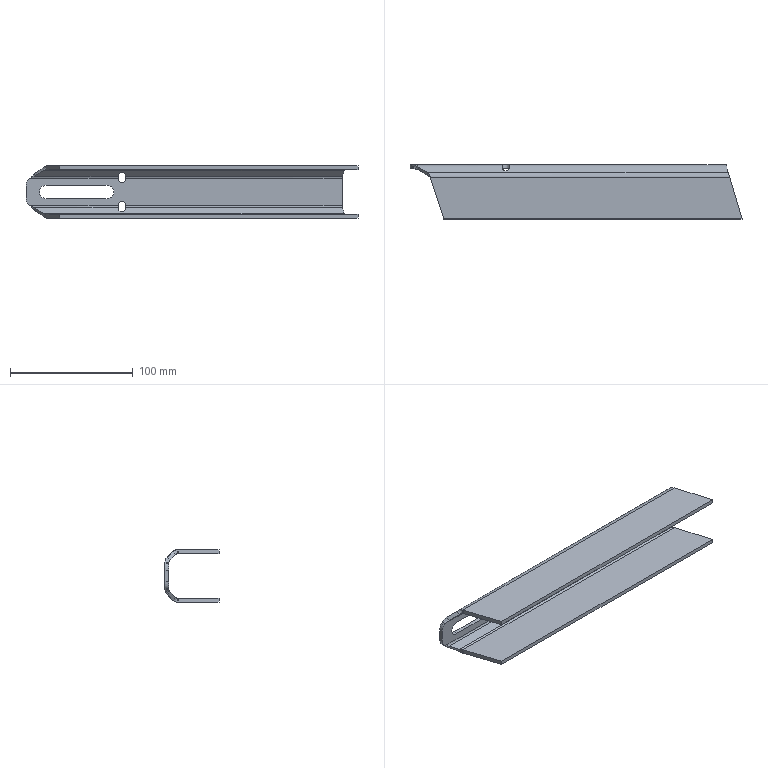Part | SolidWorks | features Fillet 2, ICE 2, FlatPattern 1, SMBaseFlange 1, SheetMetal 1, UnFold 1 | 1 solid | 69 faces | box 270.5 x 44 x 42.8 mm | volume 88895 mm3 | plane 37 | spline 16 | cylinder 16 | commonest cylinder face diameters 5 x6 11.4 x6 11 x2 16 x2